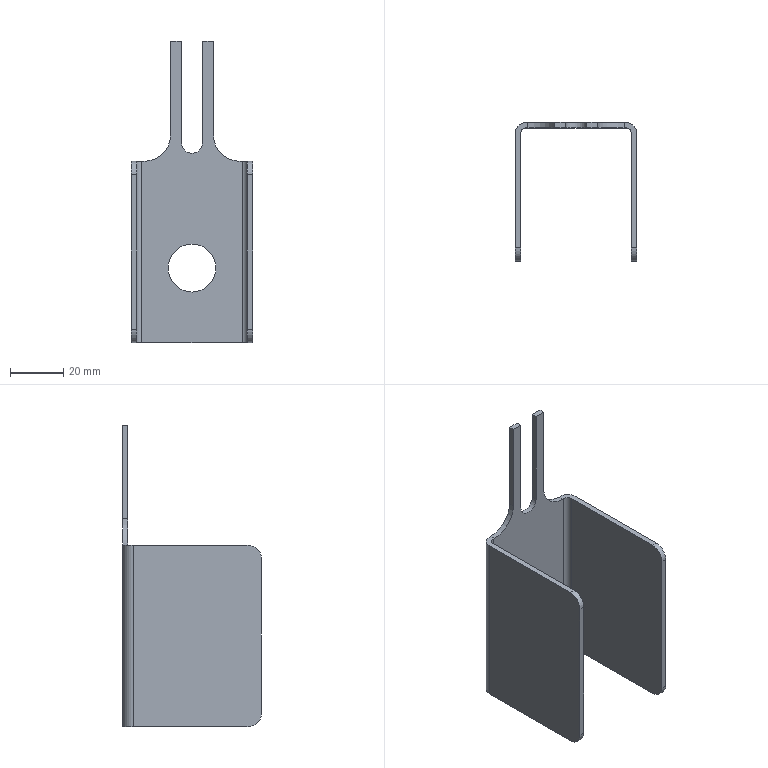Part | NX | features BREP 1 | 1 solid | 29 faces | box 45.5 x 52 x 113 mm | volume 19753 mm3 | plane 17 | cylinder 12 | commonest cylinder face diameters 10 x4 8 x3 4 x2 20 x2 18 x1
STEP:
#1=CARTESIAN_POINT('',(22.75,-50.,63.));
#2=VERTEX_POINT('',#1);
#3=CARTESIAN_POINT('',(22.75,-45.,68.));
#4=VERTEX_POINT('',#3);
#5=CARTESIAN_POINT('',(22.75,-45.,63.));
#6=DIRECTION('',(-1.,0.,0.));
#7=DIRECTION('',(0.,0.,-1.));
#8=AXIS2_PLACEMENT_3D('',#5,#6,#7);
#9=CIRCLE('',#8,5.);
#10=EDGE_CURVE('',#2,#4,#9,.T.);
#11=ORIENTED_EDGE('',*,*,#10,.F.);
#12=CARTESIAN_POINT('',(22.75,-50.,5.));
#13=VERTEX_POINT('',#12);
#14=CARTESIAN_POINT('',(22.75,-50.,113.));
#15=DIRECTION('',(0.,0.,1.));
#16=VECTOR('',#15,1000.);
#17=LINE('',#14,#16);
#18=EDGE_CURVE('',#13,#2,#17,.T.);
#19=ORIENTED_EDGE('',*,*,#18,.F.);
#20=CARTESIAN_POINT('',(22.75,-45.,0.));
#21=VERTEX_POINT('',#20);
#22=CARTESIAN_POINT('',(22.75,-45.,5.));
#23=DIRECTION('',(-1.,0.,0.));
#24=DIRECTION('',(0.,0.,1.));
#25=AXIS2_PLACEMENT_3D('',#22,#23,#24);
#26=CIRCLE('',#25,5.);
#27=EDGE_CURVE('',#21,#13,#26,.T.);
#28=ORIENTED_EDGE('',*,*,#27,.F.);
#29=CARTESIAN_POINT('',(22.75,-2.,0.));
#30=VERTEX_POINT('',#29);
#31=CARTESIAN_POINT('',(22.75,0.,0.));
#32=DIRECTION('',(0.,-1.,0.));
#33=VECTOR('',#32,1000.);
#34=LINE('',#31,#33);
#35=EDGE_CURVE('',#30,#21,#34,.T.);
#36=ORIENTED_EDGE('',*,*,#35,.F.);
#37=CARTESIAN_POINT('',(22.75,-2.,68.));
#38=VERTEX_POINT('',#37);
#39=CARTESIAN_POINT('',(22.75,-2.,113.));
#40=DIRECTION('',(0.,0.,-1.));
#41=VECTOR('',#40,1000.);
#42=LINE('',#39,#41);
#43=EDGE_CURVE('',#38,#30,#42,.T.);
#44=ORIENTED_EDGE('',*,*,#43,.F.);
#45=CARTESIAN_POINT('',(22.75,0.,68.));
#46=DIRECTION('',(0.,1.,0.));
#47=VECTOR('',#46,1000.);
#48=LINE('',#45,#47);
#49=EDGE_CURVE('',#4,#38,#48,.T.);
#50=ORIENTED_EDGE('',*,*,#49,.F.);
#51=EDGE_LOOP('',(#11,#19,#28,#36,#44,#50));
#52=FACE_BOUND('',#51,.T.);
#53=CARTESIAN_POINT('',(22.75,0.,113.));
#54=DIRECTION('',(-1.,0.,0.));
#55=DIRECTION('',(0.,1.,0.));
#56=AXIS2_PLACEMENT_3D('',#53,#54,#55);
#57=PLANE('',#56);
#58=ADVANCED_FACE('',(#52),#57,.F.);
#59=CARTESIAN_POINT('',(18.75,0.,68.));
#60=VERTEX_POINT('',#59);
#61=CARTESIAN_POINT('',(18.,0.,68.));
#62=VERTEX_POINT('',#61);
#63=CARTESIAN_POINT('',(-20.75,0.,68.));
#64=DIRECTION('',(-1.,0.,0.));
#65=VECTOR('',#64,1000.);
#66=LINE('',#63,#65);
#67=EDGE_CURVE('',#60,#62,#66,.T.);
#68=ORIENTED_EDGE('',*,*,#67,.F.);
#69=CARTESIAN_POINT('',(20.75,-2.,68.));
#70=VERTEX_POINT('',#69);
#71=CARTESIAN_POINT('',(18.75,-2.,68.));
#72=DIRECTION('',(0.,0.,-1.));
#73=DIRECTION('',(-1.,0.,0.));
#74=AXIS2_PLACEMENT_3D('',#71,#72,#73);
#75=CIRCLE('',#74,2.);
#76=EDGE_CURVE('',#60,#70,#75,.T.);
#77=ORIENTED_EDGE('',*,*,#76,.T.);
#78=CARTESIAN_POINT('',(20.75,-45.,68.));
#79=VERTEX_POINT('',#78);
#80=CARTESIAN_POINT('',(20.75,-50.,68.));
#81=DIRECTION('',(0.,-1.,0.));
#82=VECTOR('',#81,1000.);
#83=LINE('',#80,#82);
#84=EDGE_CURVE('',#70,#79,#83,.T.);
#85=ORIENTED_EDGE('',*,*,#84,.T.);
#86=CARTESIAN_POINT('',(8.,-45.,68.));
#87=DIRECTION('',(1.,0.,0.));
#88=VECTOR('',#87,1000.);
#89=LINE('',#86,#88);
#90=EDGE_CURVE('',#79,#4,#89,.T.);
#91=ORIENTED_EDGE('',*,*,#90,.T.);
#92=ORIENTED_EDGE('',*,*,#49,.T.);
#93=CARTESIAN_POINT('',(18.75,2.,68.));
#94=VERTEX_POINT('',#93);
#95=CARTESIAN_POINT('',(18.75,-2.,68.));
#96=DIRECTION('',(0.,0.,1.));
#97=DIRECTION('',(-1.,0.,0.));
#98=AXIS2_PLACEMENT_3D('',#95,#96,#97);
#99=CIRCLE('',#98,4.);
#100=EDGE_CURVE('',#38,#94,#99,.T.);
#101=ORIENTED_EDGE('',*,*,#100,.T.);
#102=CARTESIAN_POINT('',(18.,2.,68.));
#103=VERTEX_POINT('',#102);
#104=CARTESIAN_POINT('',(-20.75,2.,68.));
#105=DIRECTION('',(-1.,0.,0.));
#106=VECTOR('',#105,1000.);
#107=LINE('',#104,#106);
#108=EDGE_CURVE('',#94,#103,#107,.T.);
#109=ORIENTED_EDGE('',*,*,#108,.T.);
#110=CARTESIAN_POINT('',(18.,-50.,68.));
#111=DIRECTION('',(0.,-1.,0.));
#112=VECTOR('',#111,1000.);
#113=LINE('',#110,#112);
#114=EDGE_CURVE('',#103,#62,#113,.T.);
#115=ORIENTED_EDGE('',*,*,#114,.T.);
#116=EDGE_LOOP('',(#68,#77,#85,#91,#92,#101,#109,#115));
#117=FACE_BOUND('',#116,.T.);
#118=CARTESIAN_POINT('',(8.,-50.,68.));
#119=DIRECTION('',(0.,0.,1.));
#120=DIRECTION('',(-1.,0.,0.));
#121=AXIS2_PLACEMENT_3D('',#118,#119,#120);
#122=PLANE('',#121);
#123=ADVANCED_FACE('',(#117),#122,.T.);
#124=ORIENTED_EDGE('',*,*,#10,.T.);
#125=ORIENTED_EDGE('',*,*,#90,.F.);
#126=CARTESIAN_POINT('',(20.75,-50.,63.));
#127=VERTEX_POINT('',#126);
#128=CARTESIAN_POINT('',(20.75,-45.,63.));
#129=DIRECTION('',(1.,0.,0.));
#130=DIRECTION('',(0.,0.,-1.));
#131=AXIS2_PLACEMENT_3D('',#128,#129,#130);
#132=CIRCLE('',#131,5.);
#133=EDGE_CURVE('',#79,#127,#132,.T.);
#134=ORIENTED_EDGE('',*,*,#133,.T.);
#135=CARTESIAN_POINT('',(8.,-50.,63.));
#136=DIRECTION('',(1.,0.,0.));
#137=VECTOR('',#136,1000.);
#138=LINE('',#135,#137);
#139=EDGE_CURVE('',#127,#2,#138,.T.);
#140=ORIENTED_EDGE('',*,*,#139,.T.);
#141=EDGE_LOOP('',(#124,#125,#134,#140));
#142=FACE_BOUND('',#141,.T.);
#143=CARTESIAN_POINT('',(8.,-45.,63.));
#144=DIRECTION('',(1.,0.,0.));
#145=DIRECTION('',(0.,0.,1.));
#146=AXIS2_PLACEMENT_3D('',#143,#144,#145);
#147=CYLINDRICAL_SURFACE('',#146,5.);
#148=ADVANCED_FACE('',(#142),#147,.T.);
#149=CARTESIAN_POINT('',(20.75,-50.,5.));
#150=VERTEX_POINT('',#149);
#151=CARTESIAN_POINT('',(20.75,-50.,113.));
#152=DIRECTION('',(0.,0.,-1.));
#153=VECTOR('',#152,1000.);
#154=LINE('',#151,#153);
#155=EDGE_CURVE('',#127,#150,#154,.T.);
#156=ORIENTED_EDGE('',*,*,#155,.T.);
#157=CARTESIAN_POINT('',(22.75,-50.,5.));
#158=DIRECTION('',(1.,0.,0.));
#159=VECTOR('',#158,1000.);
#160=LINE('',#157,#159);
#161=EDGE_CURVE('',#150,#13,#160,.T.);
#162=ORIENTED_EDGE('',*,*,#161,.T.);
#163=ORIENTED_EDGE('',*,*,#18,.T.);
#164=ORIENTED_EDGE('',*,*,#139,.F.);
#165=EDGE_LOOP('',(#156,#162,#163,#164));
#166=FACE_BOUND('',#165,.T.);
#167=CARTESIAN_POINT('',(22.75,-50.,113.));
#168=DIRECTION('',(0.,-1.,0.));
#169=DIRECTION('',(0.,0.,1.));
#170=AXIS2_PLACEMENT_3D('',#167,#168,#169);
#171=PLANE('',#170);
#172=ADVANCED_FACE('',(#166),#171,.T.);
#173=CARTESIAN_POINT('',(20.75,-45.,0.));
#174=VERTEX_POINT('',#173);
#175=CARTESIAN_POINT('',(20.75,-45.,5.));
#176=DIRECTION('',(1.,0.,0.));
#177=DIRECTION('',(0.,0.,1.));
#178=AXIS2_PLACEMENT_3D('',#175,#176,#177);
#179=CIRCLE('',#178,5.);
#180=EDGE_CURVE('',#150,#174,#179,.T.);
#181=ORIENTED_EDGE('',*,*,#180,.T.);
#182=CARTESIAN_POINT('',(18.75,-45.,0.));
#183=DIRECTION('',(1.,0.,0.));
#184=VECTOR('',#183,1000.);
#185=LINE('',#182,#184);
#186=EDGE_CURVE('',#174,#21,#185,.T.);
#187=ORIENTED_EDGE('',*,*,#186,.T.);
#188=ORIENTED_EDGE('',*,*,#27,.T.);
#189=ORIENTED_EDGE('',*,*,#161,.F.);
#190=EDGE_LOOP('',(#181,#187,#188,#189));
#191=FACE_BOUND('',#190,.T.);
#192=CARTESIAN_POINT('',(18.75,-45.,5.));
#193=DIRECTION('',(-1.,0.,0.));
#194=DIRECTION('',(0.,0.,-1.));
#195=AXIS2_PLACEMENT_3D('',#192,#193,#194);
#196=CYLINDRICAL_SURFACE('',#195,5.);
#197=ADVANCED_FACE('',(#191),#196,.T.);
#198=CARTESIAN_POINT('',(20.75,-2.,0.));
#199=VERTEX_POINT('',#198);
#200=CARTESIAN_POINT('',(20.75,2.,0.));
#201=DIRECTION('',(0.,1.,0.));
#202=VECTOR('',#201,1000.);
#203=LINE('',#200,#202);
#204=EDGE_CURVE('',#174,#199,#203,.T.);
#205=ORIENTED_EDGE('',*,*,#204,.T.);
#206=CARTESIAN_POINT('',(18.75,0.,0.));
#207=VERTEX_POINT('',#206);
#208=CARTESIAN_POINT('',(18.75,-2.,0.));
#209=DIRECTION('',(0.,0.,1.));
#210=DIRECTION('',(-1.,0.,0.));
#211=AXIS2_PLACEMENT_3D('',#208,#209,#210);
#212=CIRCLE('',#211,2.);
#213=EDGE_CURVE('',#199,#207,#212,.T.);
#214=ORIENTED_EDGE('',*,*,#213,.T.);
#215=CARTESIAN_POINT('',(-18.75,0.,0.));
#216=VERTEX_POINT('',#215);
#217=CARTESIAN_POINT('',(-20.75,0.,0.));
#218=DIRECTION('',(1.,0.,0.));
#219=VECTOR('',#218,1000.);
#220=LINE('',#217,#219);
#221=EDGE_CURVE('',#216,#207,#220,.T.);
#222=ORIENTED_EDGE('',*,*,#221,.F.);
#223=CARTESIAN_POINT('',(-20.75,-2.,0.));
#224=VERTEX_POINT('',#223);
#225=CARTESIAN_POINT('',(-18.75,-2.,0.));
#226=DIRECTION('',(0.,0.,1.));
#227=DIRECTION('',(-1.,0.,0.));
#228=AXIS2_PLACEMENT_3D('',#225,#226,#227);
#229=CIRCLE('',#228,2.);
#230=EDGE_CURVE('',#216,#224,#229,.T.);
#231=ORIENTED_EDGE('',*,*,#230,.T.);
#232=CARTESIAN_POINT('',(-20.75,-45.,0.));
#233=VERTEX_POINT('',#232);
#234=CARTESIAN_POINT('',(-20.75,0.,0.));
#235=DIRECTION('',(0.,1.,0.));
#236=VECTOR('',#235,1000.);
#237=LINE('',#234,#236);
#238=EDGE_CURVE('',#233,#224,#237,.T.);
#239=ORIENTED_EDGE('',*,*,#238,.F.);
#240=CARTESIAN_POINT('',(-22.75,-45.,0.));
#241=VERTEX_POINT('',#240);
#242=CARTESIAN_POINT('',(-18.75,-45.,0.));
#243=DIRECTION('',(-1.,0.,0.));
#244=VECTOR('',#243,1000.);
#245=LINE('',#242,#244);
#246=EDGE_CURVE('',#233,#241,#245,.T.);
#247=ORIENTED_EDGE('',*,*,#246,.T.);
#248=CARTESIAN_POINT('',(-22.75,-2.,0.));
#249=VERTEX_POINT('',#248);
#250=CARTESIAN_POINT('',(-22.75,0.,0.));
#251=DIRECTION('',(0.,1.,0.));
#252=VECTOR('',#251,1000.);
#253=LINE('',#250,#252);
#254=EDGE_CURVE('',#241,#249,#253,.T.);
#255=ORIENTED_EDGE('',*,*,#254,.T.);
#256=CARTESIAN_POINT('',(-18.75,2.,0.));
#257=VERTEX_POINT('',#256);
#258=CARTESIAN_POINT('',(-18.75,-2.,0.));
#259=DIRECTION('',(0.,0.,1.));
#260=DIRECTION('',(-1.,0.,0.));
#261=AXIS2_PLACEMENT_3D('',#258,#259,#260);
#262=CIRCLE('',#261,4.);
#263=EDGE_CURVE('',#257,#249,#262,.T.);
#264=ORIENTED_EDGE('',*,*,#263,.F.);
#265=CARTESIAN_POINT('',(18.75,2.,0.));
#266=VERTEX_POINT('',#265);
#267=CARTESIAN_POINT('',(-20.75,2.,0.));
#268=DIRECTION('',(1.,0.,0.));
#269=VECTOR('',#268,1000.);
#270=LINE('',#267,#269);
#271=EDGE_CURVE('',#257,#266,#270,.T.);
#272=ORIENTED_EDGE('',*,*,#271,.T.);
#273=CARTESIAN_POINT('',(18.75,-2.,0.));
#274=DIRECTION('',(0.,0.,1.));
#275=DIRECTION('',(-1.,0.,0.));
#276=AXIS2_PLACEMENT_3D('',#273,#274,#275);
#277=CIRCLE('',#276,4.);
#278=EDGE_CURVE('',#30,#266,#277,.T.);
#279=ORIENTED_EDGE('',*,*,#278,.F.);
#280=ORIENTED_EDGE('',*,*,#35,.T.);
#281=ORIENTED_EDGE('',*,*,#186,.F.);
#282=EDGE_LOOP('',(#205,#214,#222,#231,#239,#247,#255,#264,#272,#279,#280,#281));
#283=FACE_BOUND('',#282,.T.);
#284=CARTESIAN_POINT('',(18.75,2.,0.));
#285=DIRECTION('',(0.,0.,-1.));
#286=DIRECTION('',(1.,0.,0.));
#287=AXIS2_PLACEMENT_3D('',#284,#285,#286);
#288=PLANE('',#287);
#289=ADVANCED_FACE('',(#283),#288,.T.);
#290=ORIENTED_EDGE('',*,*,#278,.T.);
#291=CARTESIAN_POINT('',(18.75,2.,113.));
#292=DIRECTION('',(0.,0.,1.));
#293=VECTOR('',#292,1000.);
#294=LINE('',#291,#293);
#295=EDGE_CURVE('',#266,#94,#294,.T.);
#296=ORIENTED_EDGE('',*,*,#295,.T.);
#297=ORIENTED_EDGE('',*,*,#100,.F.);
#298=ORIENTED_EDGE('',*,*,#43,.T.);
#299=EDGE_LOOP('',(#290,#296,#297,#298));
#300=FACE_BOUND('',#299,.T.);
#301=CARTESIAN_POINT('',(18.75,-2.,113.));
#302=DIRECTION('',(0.,0.,-1.));
#303=DIRECTION('',(1.,0.,0.));
#304=AXIS2_PLACEMENT_3D('',#301,#302,#303);
#305=CYLINDRICAL_SURFACE('',#304,4.);
#306=ADVANCED_FACE('',(#300),#305,.T.);
#307=ORIENTED_EDGE('',*,*,#76,.F.);
#308=CARTESIAN_POINT('',(18.75,0.,113.));
#309=DIRECTION('',(0.,0.,1.));
#310=VECTOR('',#309,1000.);
#311=LINE('',#308,#310);
#312=EDGE_CURVE('',#207,#60,#311,.T.);
#313=ORIENTED_EDGE('',*,*,#312,.F.);
#314=ORIENTED_EDGE('',*,*,#213,.F.);
#315=CARTESIAN_POINT('',(20.75,-2.,113.));
#316=DIRECTION('',(0.,0.,-1.));
#317=VECTOR('',#316,1000.);
#318=LINE('',#315,#317);
#319=EDGE_CURVE('',#70,#199,#318,.T.);
#320=ORIENTED_EDGE('',*,*,#319,.F.);
#321=EDGE_LOOP('',(#307,#313,#314,#320));
#322=FACE_BOUND('',#321,.T.);
#323=CARTESIAN_POINT('',(18.75,-2.,113.));
#324=DIRECTION('',(0.,0.,-1.));
#325=DIRECTION('',(1.,0.,0.));
#326=AXIS2_PLACEMENT_3D('',#323,#324,#325);
#327=CYLINDRICAL_SURFACE('',#326,2.);
#328=ADVANCED_FACE('',(#322),#327,.F.);
#329=ORIENTED_EDGE('',*,*,#114,.F.);
#330=CARTESIAN_POINT('',(8.,2.,78.));
#331=VERTEX_POINT('',#330);
#332=CARTESIAN_POINT('',(18.,2.,78.));
#333=DIRECTION('',(0.,-1.,0.));
#334=DIRECTION('',(0.,0.,-1.));
#335=AXIS2_PLACEMENT_3D('',#332,#333,#334);
#336=CIRCLE('',#335,10.);
#337=EDGE_CURVE('',#331,#103,#336,.T.);
#338=ORIENTED_EDGE('',*,*,#337,.F.);
#339=CARTESIAN_POINT('',(8.,0.,78.));
#340=VERTEX_POINT('',#339);
#341=CARTESIAN_POINT('',(8.,-50.,78.));
#342=DIRECTION('',(0.,1.,0.));
#343=VECTOR('',#342,1000.);
#344=LINE('',#341,#343);
#345=EDGE_CURVE('',#340,#331,#344,.T.);
#346=ORIENTED_EDGE('',*,*,#345,.F.);
#347=CARTESIAN_POINT('',(18.,0.,78.));
#348=DIRECTION('',(0.,1.,0.));
#349=DIRECTION('',(0.,0.,-1.));
#350=AXIS2_PLACEMENT_3D('',#347,#348,#349);
#351=CIRCLE('',#350,10.);
#352=EDGE_CURVE('',#62,#340,#351,.T.);
#353=ORIENTED_EDGE('',*,*,#352,.F.);
#354=EDGE_LOOP('',(#329,#338,#346,#353));
#355=FACE_BOUND('',#354,.T.);
#356=CARTESIAN_POINT('',(18.,-50.,78.));
#357=DIRECTION('',(0.,-1.,0.));
#358=DIRECTION('',(0.,0.,1.));
#359=AXIS2_PLACEMENT_3D('',#356,#357,#358);
#360=CYLINDRICAL_SURFACE('',#359,10.);
#361=ADVANCED_FACE('',(#355),#360,.F.);
#362=ORIENTED_EDGE('',*,*,#204,.F.);
#363=ORIENTED_EDGE('',*,*,#180,.F.);
#364=ORIENTED_EDGE('',*,*,#155,.F.);
#365=ORIENTED_EDGE('',*,*,#133,.F.);
#366=ORIENTED_EDGE('',*,*,#84,.F.);
#367=ORIENTED_EDGE('',*,*,#319,.T.);
#368=EDGE_LOOP('',(#362,#363,#364,#365,#366,#367));
#369=FACE_BOUND('',#368,.T.);
#370=CARTESIAN_POINT('',(20.75,0.,113.));
#371=DIRECTION('',(-1.,0.,0.));
#372=DIRECTION('',(0.,1.,0.));
#373=AXIS2_PLACEMENT_3D('',#370,#371,#372);
#374=PLANE('',#373);
#375=ADVANCED_FACE('',(#369),#374,.T.);
#376=CARTESIAN_POINT('',(-4.,2.,75.));
#377=VERTEX_POINT('',#376);
#378=CARTESIAN_POINT('',(-4.,2.,113.));
#379=VERTEX_POINT('',#378);
#380=CARTESIAN_POINT('',(-4.,2.,113.));
#381=DIRECTION('',(0.,0.,1.));
#382=VECTOR('',#381,1000.);
#383=LINE('',#380,#382);
#384=EDGE_CURVE('',#377,#379,#383,.T.);
#385=ORIENTED_EDGE('',*,*,#384,.F.);
#386=CARTESIAN_POINT('',(4.,2.,75.));
#387=VERTEX_POINT('',#386);
#388=CARTESIAN_POINT('',(0.,2.,75.));
#389=DIRECTION('',(0.,1.,0.));
#390=DIRECTION('',(0.,0.,1.));
#391=AXIS2_PLACEMENT_3D('',#388,#389,#390);
#392=CIRCLE('',#391,4.);
#393=EDGE_CURVE('',#387,#377,#392,.T.);
#394=ORIENTED_EDGE('',*,*,#393,.F.);
#395=CARTESIAN_POINT('',(4.,2.,113.));
#396=VERTEX_POINT('',#395);
#397=CARTESIAN_POINT('',(4.,2.,113.));
#398=DIRECTION('',(0.,0.,-1.));
#399=VECTOR('',#398,1000.);
#400=LINE('',#397,#399);
#401=EDGE_CURVE('',#396,#387,#400,.T.);
#402=ORIENTED_EDGE('',*,*,#401,.F.);
#403=CARTESIAN_POINT('',(8.,2.,113.));
#404=VERTEX_POINT('',#403);
#405=CARTESIAN_POINT('',(-20.75,2.,113.));
#406=DIRECTION('',(-1.,0.,0.));
#407=VECTOR('',#406,1000.);
#408=LINE('',#405,#407);
#409=EDGE_CURVE('',#404,#396,#408,.T.);
#410=ORIENTED_EDGE('',*,*,#409,.F.);
#411=CARTESIAN_POINT('',(8.,2.,113.));
#412=DIRECTION('',(0.,0.,1.));
#413=VECTOR('',#412,1000.);
#414=LINE('',#411,#413);
#415=EDGE_CURVE('',#331,#404,#414,.T.);
#416=ORIENTED_EDGE('',*,*,#415,.F.);
#417=ORIENTED_EDGE('',*,*,#337,.T.);
#418=ORIENTED_EDGE('',*,*,#108,.F.);
#419=ORIENTED_EDGE('',*,*,#295,.F.);
#420=ORIENTED_EDGE('',*,*,#271,.F.);
#421=CARTESIAN_POINT('',(-18.75,2.,68.));
#422=VERTEX_POINT('',#421);
#423=CARTESIAN_POINT('',(-18.75,2.,113.));
#424=DIRECTION('',(0.,0.,-1.));
#425=VECTOR('',#424,1000.);
#426=LINE('',#423,#425);
#427=EDGE_CURVE('',#422,#257,#426,.T.);
#428=ORIENTED_EDGE('',*,*,#427,.F.);
#429=CARTESIAN_POINT('',(-18.,2.,68.));
#430=VERTEX_POINT('',#429);
#431=CARTESIAN_POINT('',(-8.,2.,68.));
#432=DIRECTION('',(1.,0.,0.));
#433=VECTOR('',#432,1000.);
#434=LINE('',#431,#433);
#435=EDGE_CURVE('',#422,#430,#434,.T.);
#436=ORIENTED_EDGE('',*,*,#435,.T.);
#437=CARTESIAN_POINT('',(-8.,2.,78.));
#438=VERTEX_POINT('',#437);
#439=CARTESIAN_POINT('',(-18.,2.,78.));
#440=DIRECTION('',(0.,1.,0.));
#441=DIRECTION('',(0.,0.,-1.));
#442=AXIS2_PLACEMENT_3D('',#439,#440,#441);
#443=CIRCLE('',#442,10.);
#444=EDGE_CURVE('',#438,#430,#443,.T.);
#445=ORIENTED_EDGE('',*,*,#444,.F.);
#446=CARTESIAN_POINT('',(-8.,2.,113.));
#447=VERTEX_POINT('',#446);
#448=CARTESIAN_POINT('',(-8.,2.,113.));
#449=DIRECTION('',(0.,0.,-1.));
#450=VECTOR('',#449,1000.);
#451=LINE('',#448,#450);
#452=EDGE_CURVE('',#447,#438,#451,.T.);
#453=ORIENTED_EDGE('',*,*,#452,.F.);
#454=CARTESIAN_POINT('',(-20.75,2.,113.));
#455=DIRECTION('',(-1.,0.,0.));
#456=VECTOR('',#455,1000.);
#457=LINE('',#454,#456);
#458=EDGE_CURVE('',#379,#447,#457,.T.);
#459=ORIENTED_EDGE('',*,*,#458,.F.);
#460=EDGE_LOOP('',(#385,#394,#402,#410,#416,#417,#418,#419,#420,#428,#436,#445,#453,#459));
#461=FACE_BOUND('',#460,.T.);
#462=CARTESIAN_POINT('',(0.,2.,37.));
#463=VERTEX_POINT('',#462);
#464=CARTESIAN_POINT('',(0.,2.,28.));
#465=DIRECTION('',(0.,1.,0.));
#466=DIRECTION('',(0.,0.,1.));
#467=AXIS2_PLACEMENT_3D('',#464,#465,#466);
#468=CIRCLE('',#467,9.);
#469=EDGE_CURVE('',#463,#463,#468,.T.);
#470=ORIENTED_EDGE('',*,*,#469,.F.);
#471=EDGE_LOOP('',(#470));
#472=FACE_BOUND('',#471,.T.);
#473=CARTESIAN_POINT('',(-20.75,2.,113.));
#474=DIRECTION('',(0.,-1.,0.));
#475=DIRECTION('',(0.,0.,1.));
#476=AXIS2_PLACEMENT_3D('',#473,#474,#475);
#477=PLANE('',#476);
#478=ADVANCED_FACE('',(#461,#472),#477,.F.);
#479=CARTESIAN_POINT('',(4.,0.,113.));
#480=VERTEX_POINT('',#479);
#481=CARTESIAN_POINT('',(4.,0.,75.));
#482=VERTEX_POINT('',#481);
#483=CARTESIAN_POINT('',(4.,0.,113.));
#484=DIRECTION('',(0.,0.,-1.));
#485=VECTOR('',#484,1000.);
#486=LINE('',#483,#485);
#487=EDGE_CURVE('',#480,#482,#486,.T.);
#488=ORIENTED_EDGE('',*,*,#487,.T.);
#489=CARTESIAN_POINT('',(-4.,0.,75.));
#490=VERTEX_POINT('',#489);
#491=CARTESIAN_POINT('',(0.,0.,75.));
#492=DIRECTION('',(0.,1.,0.));
#493=DIRECTION('',(0.,0.,1.));
#494=AXIS2_PLACEMENT_3D('',#491,#492,#493);
#495=CIRCLE('',#494,4.);
#496=EDGE_CURVE('',#482,#490,#495,.T.);
#497=ORIENTED_EDGE('',*,*,#496,.T.);
#498=CARTESIAN_POINT('',(-4.,0.,113.));
#499=VERTEX_POINT('',#498);
#500=CARTESIAN_POINT('',(-4.,0.,113.));
#501=DIRECTION('',(0.,0.,1.));
#502=VECTOR('',#501,1000.);
#503=LINE('',#500,#502);
#504=EDGE_CURVE('',#490,#499,#503,.T.);
#505=ORIENTED_EDGE('',*,*,#504,.T.);
#506=CARTESIAN_POINT('',(-8.,0.,113.));
#507=VERTEX_POINT('',#506);
#508=CARTESIAN_POINT('',(-20.75,0.,113.));
#509=DIRECTION('',(-1.,0.,0.));
#510=VECTOR('',#509,1000.);
#511=LINE('',#508,#510);
#512=EDGE_CURVE('',#499,#507,#511,.T.);
#513=ORIENTED_EDGE('',*,*,#512,.T.);
#514=CARTESIAN_POINT('',(-8.,0.,78.));
#515=VERTEX_POINT('',#514);
#516=CARTESIAN_POINT('',(-8.,0.,113.));
#517=DIRECTION('',(0.,0.,-1.));
#518=VECTOR('',#517,1000.);
#519=LINE('',#516,#518);
#520=EDGE_CURVE('',#507,#515,#519,.T.);
#521=ORIENTED_EDGE('',*,*,#520,.T.);
#522=CARTESIAN_POINT('',(-18.,0.,68.));
#523=VERTEX_POINT('',#522);
#524=CARTESIAN_POINT('',(-18.,0.,78.));
#525=DIRECTION('',(0.,1.,0.));
#526=DIRECTION('',(0.,0.,-1.));
#527=AXIS2_PLACEMENT_3D('',#524,#525,#526);
#528=CIRCLE('',#527,10.);
#529=EDGE_CURVE('',#515,#523,#528,.T.);
#530=ORIENTED_EDGE('',*,*,#529,.T.);
#531=CARTESIAN_POINT('',(-18.75,0.,68.));
#532=VERTEX_POINT('',#531);
#533=CARTESIAN_POINT('',(-8.,0.,68.));
#534=DIRECTION('',(-1.,0.,0.));
#535=VECTOR('',#534,1000.);
#536=LINE('',#533,#535);
#537=EDGE_CURVE('',#523,#532,#536,.T.);
#538=ORIENTED_EDGE('',*,*,#537,.T.);
#539=CARTESIAN_POINT('',(-18.75,0.,113.));
#540=DIRECTION('',(0.,0.,-1.));
#541=VECTOR('',#540,1000.);
#542=LINE('',#539,#541);
#543=EDGE_CURVE('',#532,#216,#542,.T.);
#544=ORIENTED_EDGE('',*,*,#543,.T.);
#545=ORIENTED_EDGE('',*,*,#221,.T.);
#546=ORIENTED_EDGE('',*,*,#312,.T.);
#547=ORIENTED_EDGE('',*,*,#67,.T.);
#548=ORIENTED_EDGE('',*,*,#352,.T.);
#549=CARTESIAN_POINT('',(8.,0.,113.));
#550=VERTEX_POINT('',#549);
#551=CARTESIAN_POINT('',(8.,0.,113.));
#552=DIRECTION('',(0.,0.,1.));
#553=VECTOR('',#552,1000.);
#554=LINE('',#551,#553);
#555=EDGE_CURVE('',#340,#550,#554,.T.);
#556=ORIENTED_EDGE('',*,*,#555,.T.);
#557=CARTESIAN_POINT('',(-20.75,0.,113.));
#558=DIRECTION('',(-1.,0.,0.));
#559=VECTOR('',#558,1000.);
#560=LINE('',#557,#559);
#561=EDGE_CURVE('',#550,#480,#560,.T.);
#562=ORIENTED_EDGE('',*,*,#561,.T.);
#563=EDGE_LOOP('',(#488,#497,#505,#513,#521,#530,#538,#544,#545,#546,#547,#548,#556,#562));
#564=FACE_BOUND('',#563,.T.);
#565=CARTESIAN_POINT('',(0.,0.,37.));
#566=VERTEX_POINT('',#565);
#567=CARTESIAN_POINT('',(0.,0.,28.));
#568=DIRECTION('',(0.,1.,0.));
#569=DIRECTION('',(0.,0.,1.));
#570=AXIS2_PLACEMENT_3D('',#567,#568,#569);
#571=CIRCLE('',#570,9.);
#572=EDGE_CURVE('',#566,#566,#571,.T.);
#573=ORIENTED_EDGE('',*,*,#572,.T.);
#574=EDGE_LOOP('',(#573));
#575=FACE_BOUND('',#574,.T.);
#576=CARTESIAN_POINT('',(-20.75,0.,113.));
#577=DIRECTION('',(0.,-1.,0.));
#578=DIRECTION('',(0.,0.,1.));
#579=AXIS2_PLACEMENT_3D('',#576,#577,#578);
#580=PLANE('',#579);
#581=ADVANCED_FACE('',(#564,#575),#580,.T.);
#582=ORIENTED_EDGE('',*,*,#415,.T.);
#583=CARTESIAN_POINT('',(8.,-50.,113.));
#584=DIRECTION('',(0.,-1.,0.));
#585=VECTOR('',#584,1000.);
#586=LINE('',#583,#585);
#587=EDGE_CURVE('',#404,#550,#586,.T.);
#588=ORIENTED_EDGE('',*,*,#587,.T.);
#589=ORIENTED_EDGE('',*,*,#555,.F.);
#590=ORIENTED_EDGE('',*,*,#345,.T.);
#591=EDGE_LOOP('',(#582,#588,#589,#590));
#592=FACE_BOUND('',#591,.T.);
#593=CARTESIAN_POINT('',(8.,-50.,68.));
#594=DIRECTION('',(1.,0.,0.));
#595=DIRECTION('',(0.,0.,1.));
#596=AXIS2_PLACEMENT_3D('',#593,#594,#595);
#597=PLANE('',#596);
#598=ADVANCED_FACE('',(#592),#597,.T.);
#599=CARTESIAN_POINT('',(-8.,-2.,113.));
#600=DIRECTION('',(0.,-1.,0.));
#601=VECTOR('',#600,1000.);
#602=LINE('',#599,#601);
#603=EDGE_CURVE('',#447,#507,#602,.T.);
#604=ORIENTED_EDGE('',*,*,#603,.T.);
#605=ORIENTED_EDGE('',*,*,#512,.F.);
#606=CARTESIAN_POINT('',(-4.,-2.,113.));
#607=DIRECTION('',(0.,1.,0.));
#608=VECTOR('',#607,1000.);
#609=LINE('',#606,#608);
#610=EDGE_CURVE('',#499,#379,#609,.T.);
#611=ORIENTED_EDGE('',*,*,#610,.T.);
#612=ORIENTED_EDGE('',*,*,#458,.T.);
#613=EDGE_LOOP('',(#604,#605,#611,#612));
#614=FACE_BOUND('',#613,.T.);
#615=CARTESIAN_POINT('',(22.75,-2.,113.));
#616=DIRECTION('',(0.,0.,1.));
#617=DIRECTION('',(-1.,0.,0.));
#618=AXIS2_PLACEMENT_3D('',#615,#616,#617);
#619=PLANE('',#618);
#620=ADVANCED_FACE('',(#614),#619,.T.);
#621=CARTESIAN_POINT('',(-4.,-8.,75.));
#622=DIRECTION('',(0.,-1.,0.));
#623=VECTOR('',#622,1000.);
#624=LINE('',#621,#623);
#625=EDGE_CURVE('',#377,#490,#624,.T.);
#626=ORIENTED_EDGE('',*,*,#625,.F.);
#627=ORIENTED_EDGE('',*,*,#384,.T.);
#628=ORIENTED_EDGE('',*,*,#610,.F.);
#629=ORIENTED_EDGE('',*,*,#504,.F.);
#630=EDGE_LOOP('',(#626,#627,#628,#629));
#631=FACE_BOUND('',#630,.T.);
#632=CARTESIAN_POINT('',(-4.,-8.,113.));
#633=DIRECTION('',(-1.,0.,0.));
#634=DIRECTION('',(0.,0.,-1.));
#635=AXIS2_PLACEMENT_3D('',#632,#633,#634);
#636=PLANE('',#635);
#637=ADVANCED_FACE('',(#631),#636,.F.);
#638=CARTESIAN_POINT('',(4.,-8.,75.));
#639=DIRECTION('',(0.,-1.,0.));
#640=VECTOR('',#639,1000.);
#641=LINE('',#638,#640);
#642=EDGE_CURVE('',#387,#482,#641,.T.);
#643=ORIENTED_EDGE('',*,*,#642,.F.);
#644=ORIENTED_EDGE('',*,*,#393,.T.);
#645=ORIENTED_EDGE('',*,*,#625,.T.);
#646=ORIENTED_EDGE('',*,*,#496,.F.);
#647=EDGE_LOOP('',(#643,#644,#645,#646));
#648=FACE_BOUND('',#647,.T.);
#649=CARTESIAN_POINT('',(0.,-8.,75.));
#650=DIRECTION('',(0.,1.,0.));
#651=DIRECTION('',(0.,0.,-1.));
#652=AXIS2_PLACEMENT_3D('',#649,#650,#651);
#653=CYLINDRICAL_SURFACE('',#652,4.);
#654=ADVANCED_FACE('',(#648),#653,.F.);
#655=CARTESIAN_POINT('',(4.,-8.,113.));
#656=DIRECTION('',(0.,-1.,0.));
#657=VECTOR('',#656,1000.);
#658=LINE('',#655,#657);
#659=EDGE_CURVE('',#396,#480,#658,.T.);
#660=ORIENTED_EDGE('',*,*,#659,.F.);
#661=ORIENTED_EDGE('',*,*,#401,.T.);
#662=ORIENTED_EDGE('',*,*,#642,.T.);
#663=ORIENTED_EDGE('',*,*,#487,.F.);
#664=EDGE_LOOP('',(#660,#661,#662,#663));
#665=FACE_BOUND('',#664,.T.);
#666=CARTESIAN_POINT('',(4.,-8.,113.));
#667=DIRECTION('',(1.,0.,0.));
#668=DIRECTION('',(0.,0.,1.));
#669=AXIS2_PLACEMENT_3D('',#666,#667,#668);
#670=PLANE('',#669);
#671=ADVANCED_FACE('',(#665),#670,.F.);
#672=ORIENTED_EDGE('',*,*,#587,.F.);
#673=ORIENTED_EDGE('',*,*,#409,.T.);
#674=ORIENTED_EDGE('',*,*,#659,.T.);
#675=ORIENTED_EDGE('',*,*,#561,.F.);
#676=EDGE_LOOP('',(#672,#673,#674,#675));
#677=FACE_BOUND('',#676,.T.);
#678=CARTESIAN_POINT('',(22.75,-2.,113.));
#679=DIRECTION('',(0.,0.,1.));
#680=DIRECTION('',(-1.,0.,0.));
#681=AXIS2_PLACEMENT_3D('',#678,#679,#680);
#682=PLANE('',#681);
#683=ADVANCED_FACE('',(#677),#682,.T.);
#684=ORIENTED_EDGE('',*,*,#427,.T.);
#685=ORIENTED_EDGE('',*,*,#263,.T.);
#686=CARTESIAN_POINT('',(-22.75,-2.,68.));
#687=VERTEX_POINT('',#686);
#688=CARTESIAN_POINT('',(-22.75,-2.,113.));
#689=DIRECTION('',(0.,0.,1.));
#690=VECTOR('',#689,1000.);
#691=LINE('',#688,#690);
#692=EDGE_CURVE('',#249,#687,#691,.T.);
#693=ORIENTED_EDGE('',*,*,#692,.T.);
#694=CARTESIAN_POINT('',(-18.75,-2.,68.));
#695=DIRECTION('',(0.,0.,-1.));
#696=DIRECTION('',(-1.,0.,0.));
#697=AXIS2_PLACEMENT_3D('',#694,#695,#696);
#698=CIRCLE('',#697,4.);
#699=EDGE_CURVE('',#687,#422,#698,.T.);
#700=ORIENTED_EDGE('',*,*,#699,.T.);
#701=EDGE_LOOP('',(#684,#685,#693,#700));
#702=FACE_BOUND('',#701,.T.);
#703=CARTESIAN_POINT('',(-18.75,-2.,113.));
#704=DIRECTION('',(0.,0.,-1.));
#705=DIRECTION('',(1.,0.,0.));
#706=AXIS2_PLACEMENT_3D('',#703,#704,#705);
#707=CYLINDRICAL_SURFACE('',#706,4.);
#708=ADVANCED_FACE('',(#702),#707,.T.);
#709=CARTESIAN_POINT('',(-8.,-50.,78.));
#710=DIRECTION('',(0.,-1.,0.));
#711=VECTOR('',#710,1000.);
#712=LINE('',#709,#711);
#713=EDGE_CURVE('',#438,#515,#712,.T.);
#714=ORIENTED_EDGE('',*,*,#713,.F.);
#715=ORIENTED_EDGE('',*,*,#444,.T.);
#716=CARTESIAN_POINT('',(-18.,-50.,68.));
#717=DIRECTION('',(0.,1.,0.));
#718=VECTOR('',#717,1000.);
#719=LINE('',#716,#718);
#720=EDGE_CURVE('',#523,#430,#719,.T.);
#721=ORIENTED_EDGE('',*,*,#720,.F.);
#722=ORIENTED_EDGE('',*,*,#529,.F.);
#723=EDGE_LOOP('',(#714,#715,#721,#722));
#724=FACE_BOUND('',#723,.T.);
#725=CARTESIAN_POINT('',(-18.,-50.,78.));
#726=DIRECTION('',(0.,-1.,0.));
#727=DIRECTION('',(0.,0.,1.));
#728=AXIS2_PLACEMENT_3D('',#725,#726,#727);
#729=CYLINDRICAL_SURFACE('',#728,10.);
#730=ADVANCED_FACE('',(#724),#729,.F.);
#731=ORIENTED_EDGE('',*,*,#713,.T.);
#732=ORIENTED_EDGE('',*,*,#520,.F.);
#733=ORIENTED_EDGE('',*,*,#603,.F.);
#734=ORIENTED_EDGE('',*,*,#452,.T.);
#735=EDGE_LOOP('',(#731,#732,#733,#734));
#736=FACE_BOUND('',#735,.T.);
#737=CARTESIAN_POINT('',(-8.,-50.,68.));
#738=DIRECTION('',(1.,0.,0.));
#739=DIRECTION('',(0.,0.,1.));
#740=AXIS2_PLACEMENT_3D('',#737,#738,#739);
#741=PLANE('',#740);
#742=ADVANCED_FACE('',(#736),#741,.F.);
#743=ORIENTED_EDGE('',*,*,#572,.F.);
#744=EDGE_LOOP('',(#743));
#745=FACE_BOUND('',#744,.T.);
#746=ORIENTED_EDGE('',*,*,#469,.T.);
#747=EDGE_LOOP('',(#746));
#748=FACE_BOUND('',#747,.T.);
#749=CARTESIAN_POINT('',(0.,-8.,28.));
#750=DIRECTION('',(0.,1.,0.));
#751=DIRECTION('',(0.,0.,-1.));
#752=AXIS2_PLACEMENT_3D('',#749,#750,#751);
#753=CYLINDRICAL_SURFACE('',#752,9.);
#754=ADVANCED_FACE('',(#745,#748),#753,.F.);
#755=CARTESIAN_POINT('',(-20.75,-2.,68.));
#756=VERTEX_POINT('',#755);
#757=CARTESIAN_POINT('',(-20.75,-2.,113.));
#758=DIRECTION('',(0.,0.,1.));
#759=VECTOR('',#758,1000.);
#760=LINE('',#757,#759);
#761=EDGE_CURVE('',#224,#756,#760,.T.);
#762=ORIENTED_EDGE('',*,*,#761,.F.);
#763=ORIENTED_EDGE('',*,*,#230,.F.);
#764=ORIENTED_EDGE('',*,*,#543,.F.);
#765=CARTESIAN_POINT('',(-18.75,-2.,68.));
#766=DIRECTION('',(0.,0.,-1.));
#767=DIRECTION('',(-1.,0.,0.));
#768=AXIS2_PLACEMENT_3D('',#765,#766,#767);
#769=CIRCLE('',#768,2.);
#770=EDGE_CURVE('',#756,#532,#769,.T.);
#771=ORIENTED_EDGE('',*,*,#770,.F.);
#772=EDGE_LOOP('',(#762,#763,#764,#771));
#773=FACE_BOUND('',#772,.T.);
#774=CARTESIAN_POINT('',(-18.75,-2.,113.));
#775=DIRECTION('',(0.,0.,-1.));
#776=DIRECTION('',(1.,0.,0.));
#777=AXIS2_PLACEMENT_3D('',#774,#775,#776);
#778=CYLINDRICAL_SURFACE('',#777,2.);
#779=ADVANCED_FACE('',(#773),#778,.F.);
#780=CARTESIAN_POINT('',(-20.75,-45.,68.));
#781=VERTEX_POINT('',#780);
#782=CARTESIAN_POINT('',(-22.75,-45.,68.));
#783=VERTEX_POINT('',#782);
#784=CARTESIAN_POINT('',(-8.,-45.,68.));
#785=DIRECTION('',(-1.,0.,0.));
#786=VECTOR('',#785,1000.);
#787=LINE('',#784,#786);
#788=EDGE_CURVE('',#781,#783,#787,.T.);
#789=ORIENTED_EDGE('',*,*,#788,.F.);
#790=CARTESIAN_POINT('',(-20.75,-50.,68.));
#791=DIRECTION('',(0.,-1.,0.));
#792=VECTOR('',#791,1000.);
#793=LINE('',#790,#792);
#794=EDGE_CURVE('',#756,#781,#793,.T.);
#795=ORIENTED_EDGE('',*,*,#794,.F.);
#796=ORIENTED_EDGE('',*,*,#770,.T.);
#797=ORIENTED_EDGE('',*,*,#537,.F.);
#798=ORIENTED_EDGE('',*,*,#720,.T.);
#799=ORIENTED_EDGE('',*,*,#435,.F.);
#800=ORIENTED_EDGE('',*,*,#699,.F.);
#801=CARTESIAN_POINT('',(-22.75,-50.,68.));
#802=DIRECTION('',(0.,1.,0.));
#803=VECTOR('',#802,1000.);
#804=LINE('',#801,#803);
#805=EDGE_CURVE('',#783,#687,#804,.T.);
#806=ORIENTED_EDGE('',*,*,#805,.F.);
#807=EDGE_LOOP('',(#789,#795,#796,#797,#798,#799,#800,#806));
#808=FACE_BOUND('',#807,.T.);
#809=CARTESIAN_POINT('',(-8.,-50.,68.));
#810=DIRECTION('',(0.,0.,-1.));
#811=DIRECTION('',(1.,0.,0.));
#812=AXIS2_PLACEMENT_3D('',#809,#810,#811);
#813=PLANE('',#812);
#814=ADVANCED_FACE('',(#808),#813,.F.);
#815=CARTESIAN_POINT('',(-22.75,-50.,63.));
#816=VERTEX_POINT('',#815);
#817=CARTESIAN_POINT('',(-22.75,-45.,63.));
#818=DIRECTION('',(1.,0.,0.));
#819=DIRECTION('',(0.,0.,-1.));
#820=AXIS2_PLACEMENT_3D('',#817,#818,#819);
#821=CIRCLE('',#820,5.);
#822=EDGE_CURVE('',#783,#816,#821,.T.);
#823=ORIENTED_EDGE('',*,*,#822,.F.);
#824=ORIENTED_EDGE('',*,*,#805,.T.);
#825=ORIENTED_EDGE('',*,*,#692,.F.);
#826=ORIENTED_EDGE('',*,*,#254,.F.);
#827=CARTESIAN_POINT('',(-22.75,-50.,5.));
#828=VERTEX_POINT('',#827);
#829=CARTESIAN_POINT('',(-22.75,-45.,5.));
#830=DIRECTION('',(1.,0.,0.));
#831=DIRECTION('',(0.,0.,1.));
#832=AXIS2_PLACEMENT_3D('',#829,#830,#831);
#833=CIRCLE('',#832,5.);
#834=EDGE_CURVE('',#828,#241,#833,.T.);
#835=ORIENTED_EDGE('',*,*,#834,.F.);
#836=CARTESIAN_POINT('',(-22.75,-50.,113.));
#837=DIRECTION('',(0.,0.,-1.));
#838=VECTOR('',#837,1000.);
#839=LINE('',#836,#838);
#840=EDGE_CURVE('',#816,#828,#839,.T.);
#841=ORIENTED_EDGE('',*,*,#840,.F.);
#842=EDGE_LOOP('',(#823,#824,#825,#826,#835,#841));
#843=FACE_BOUND('',#842,.T.);
#844=CARTESIAN_POINT('',(-22.75,0.,113.));
#845=DIRECTION('',(1.,0.,0.));
#846=DIRECTION('',(0.,-1.,0.));
#847=AXIS2_PLACEMENT_3D('',#844,#845,#846);
#848=PLANE('',#847);
#849=ADVANCED_FACE('',(#843),#848,.F.);
#850=ORIENTED_EDGE('',*,*,#238,.T.);
#851=ORIENTED_EDGE('',*,*,#761,.T.);
#852=ORIENTED_EDGE('',*,*,#794,.T.);
#853=CARTESIAN_POINT('',(-20.75,-50.,63.));
#854=VERTEX_POINT('',#853);
#855=CARTESIAN_POINT('',(-20.75,-45.,63.));
#856=DIRECTION('',(1.,0.,0.));
#857=DIRECTION('',(0.,0.,-1.));
#858=AXIS2_PLACEMENT_3D('',#855,#856,#857);
#859=CIRCLE('',#858,5.);
#860=EDGE_CURVE('',#781,#854,#859,.T.);
#861=ORIENTED_EDGE('',*,*,#860,.T.);
#862=CARTESIAN_POINT('',(-20.75,-50.,5.));
#863=VERTEX_POINT('',#862);
#864=CARTESIAN_POINT('',(-20.75,-50.,113.));
#865=DIRECTION('',(0.,0.,-1.));
#866=VECTOR('',#865,1000.);
#867=LINE('',#864,#866);
#868=EDGE_CURVE('',#854,#863,#867,.T.);
#869=ORIENTED_EDGE('',*,*,#868,.T.);
#870=CARTESIAN_POINT('',(-20.75,-45.,5.));
#871=DIRECTION('',(1.,0.,0.));
#872=DIRECTION('',(0.,0.,1.));
#873=AXIS2_PLACEMENT_3D('',#870,#871,#872);
#874=CIRCLE('',#873,5.);
#875=EDGE_CURVE('',#863,#233,#874,.T.);
#876=ORIENTED_EDGE('',*,*,#875,.T.);
#877=EDGE_LOOP('',(#850,#851,#852,#861,#869,#876));
#878=FACE_BOUND('',#877,.T.);
#879=CARTESIAN_POINT('',(-20.75,0.,113.));
#880=DIRECTION('',(1.,0.,0.));
#881=DIRECTION('',(0.,-1.,0.));
#882=AXIS2_PLACEMENT_3D('',#879,#880,#881);
#883=PLANE('',#882);
#884=ADVANCED_FACE('',(#878),#883,.T.);
#885=ORIENTED_EDGE('',*,*,#822,.T.);
#886=CARTESIAN_POINT('',(-20.75,-50.,63.));
#887=DIRECTION('',(1.,0.,0.));
#888=VECTOR('',#887,1000.);
#889=LINE('',#886,#888);
#890=EDGE_CURVE('',#816,#854,#889,.T.);
#891=ORIENTED_EDGE('',*,*,#890,.T.);
#892=ORIENTED_EDGE('',*,*,#860,.F.);
#893=ORIENTED_EDGE('',*,*,#788,.T.);
#894=EDGE_LOOP('',(#885,#891,#892,#893));
#895=FACE_BOUND('',#894,.T.);
#896=CARTESIAN_POINT('',(-20.75,-45.,63.));
#897=DIRECTION('',(1.,0.,0.));
#898=DIRECTION('',(0.,0.,1.));
#899=AXIS2_PLACEMENT_3D('',#896,#897,#898);
#900=CYLINDRICAL_SURFACE('',#899,5.);
#901=ADVANCED_FACE('',(#895),#900,.T.);
#902=ORIENTED_EDGE('',*,*,#840,.T.);
#903=CARTESIAN_POINT('',(-20.75,-50.,5.));
#904=DIRECTION('',(1.,0.,0.));
#905=VECTOR('',#904,1000.);
#906=LINE('',#903,#905);
#907=EDGE_CURVE('',#828,#863,#906,.T.);
#908=ORIENTED_EDGE('',*,*,#907,.T.);
#909=ORIENTED_EDGE('',*,*,#868,.F.);
#910=ORIENTED_EDGE('',*,*,#890,.F.);
#911=EDGE_LOOP('',(#902,#908,#909,#910));
#912=FACE_BOUND('',#911,.T.);
#913=CARTESIAN_POINT('',(-20.75,-50.,113.));
#914=DIRECTION('',(0.,-1.,0.));
#915=DIRECTION('',(0.,0.,1.));
#916=AXIS2_PLACEMENT_3D('',#913,#914,#915);
#917=PLANE('',#916);
#918=ADVANCED_FACE('',(#912),#917,.T.);
#919=ORIENTED_EDGE('',*,*,#834,.T.);
#920=ORIENTED_EDGE('',*,*,#246,.F.);
#921=ORIENTED_EDGE('',*,*,#875,.F.);
#922=ORIENTED_EDGE('',*,*,#907,.F.);
#923=EDGE_LOOP('',(#919,#920,#921,#922));
#924=FACE_BOUND('',#923,.T.);
#925=CARTESIAN_POINT('',(-18.75,-45.,5.));
#926=DIRECTION('',(-1.,0.,0.));
#927=DIRECTION('',(0.,0.,-1.));
#928=AXIS2_PLACEMENT_3D('',#925,#926,#927);
#929=CYLINDRICAL_SURFACE('',#928,5.);
#930=ADVANCED_FACE('',(#924),#929,.T.);
#931=CLOSED_SHELL('',(#58,#123,#148,#172,#197,#289,#306,#328,#361,#375,#478,#581,#598,#620,#637,#654,#671,#683,#708,#730,#742,#754,#779,#814,#849,#884,#901,#918,#930));
#932=MANIFOLD_SOLID_BREP('',#931);
#933=(LENGTH_UNIT()NAMED_UNIT(*)SI_UNIT(.MILLI.,.METRE.));
#934=UNCERTAINTY_MEASURE_WITH_UNIT(LENGTH_MEASURE(0.00001),#933,'','');
#935=(NAMED_UNIT(*)PLANE_ANGLE_UNIT()SI_UNIT($,.RADIAN.));
#936=(NAMED_UNIT(*)SI_UNIT($,.STERADIAN.)SOLID_ANGLE_UNIT());
#937=(GEOMETRIC_REPRESENTATION_CONTEXT(3)GLOBAL_UNCERTAINTY_ASSIGNED_CONTEXT((#934))GLOBAL_UNIT_ASSIGNED_CONTEXT((#933,#935,#936))REPRESENTATION_CONTEXT('',''));
#938=ADVANCED_BREP_SHAPE_REPRESENTATION('',(#932),#937);